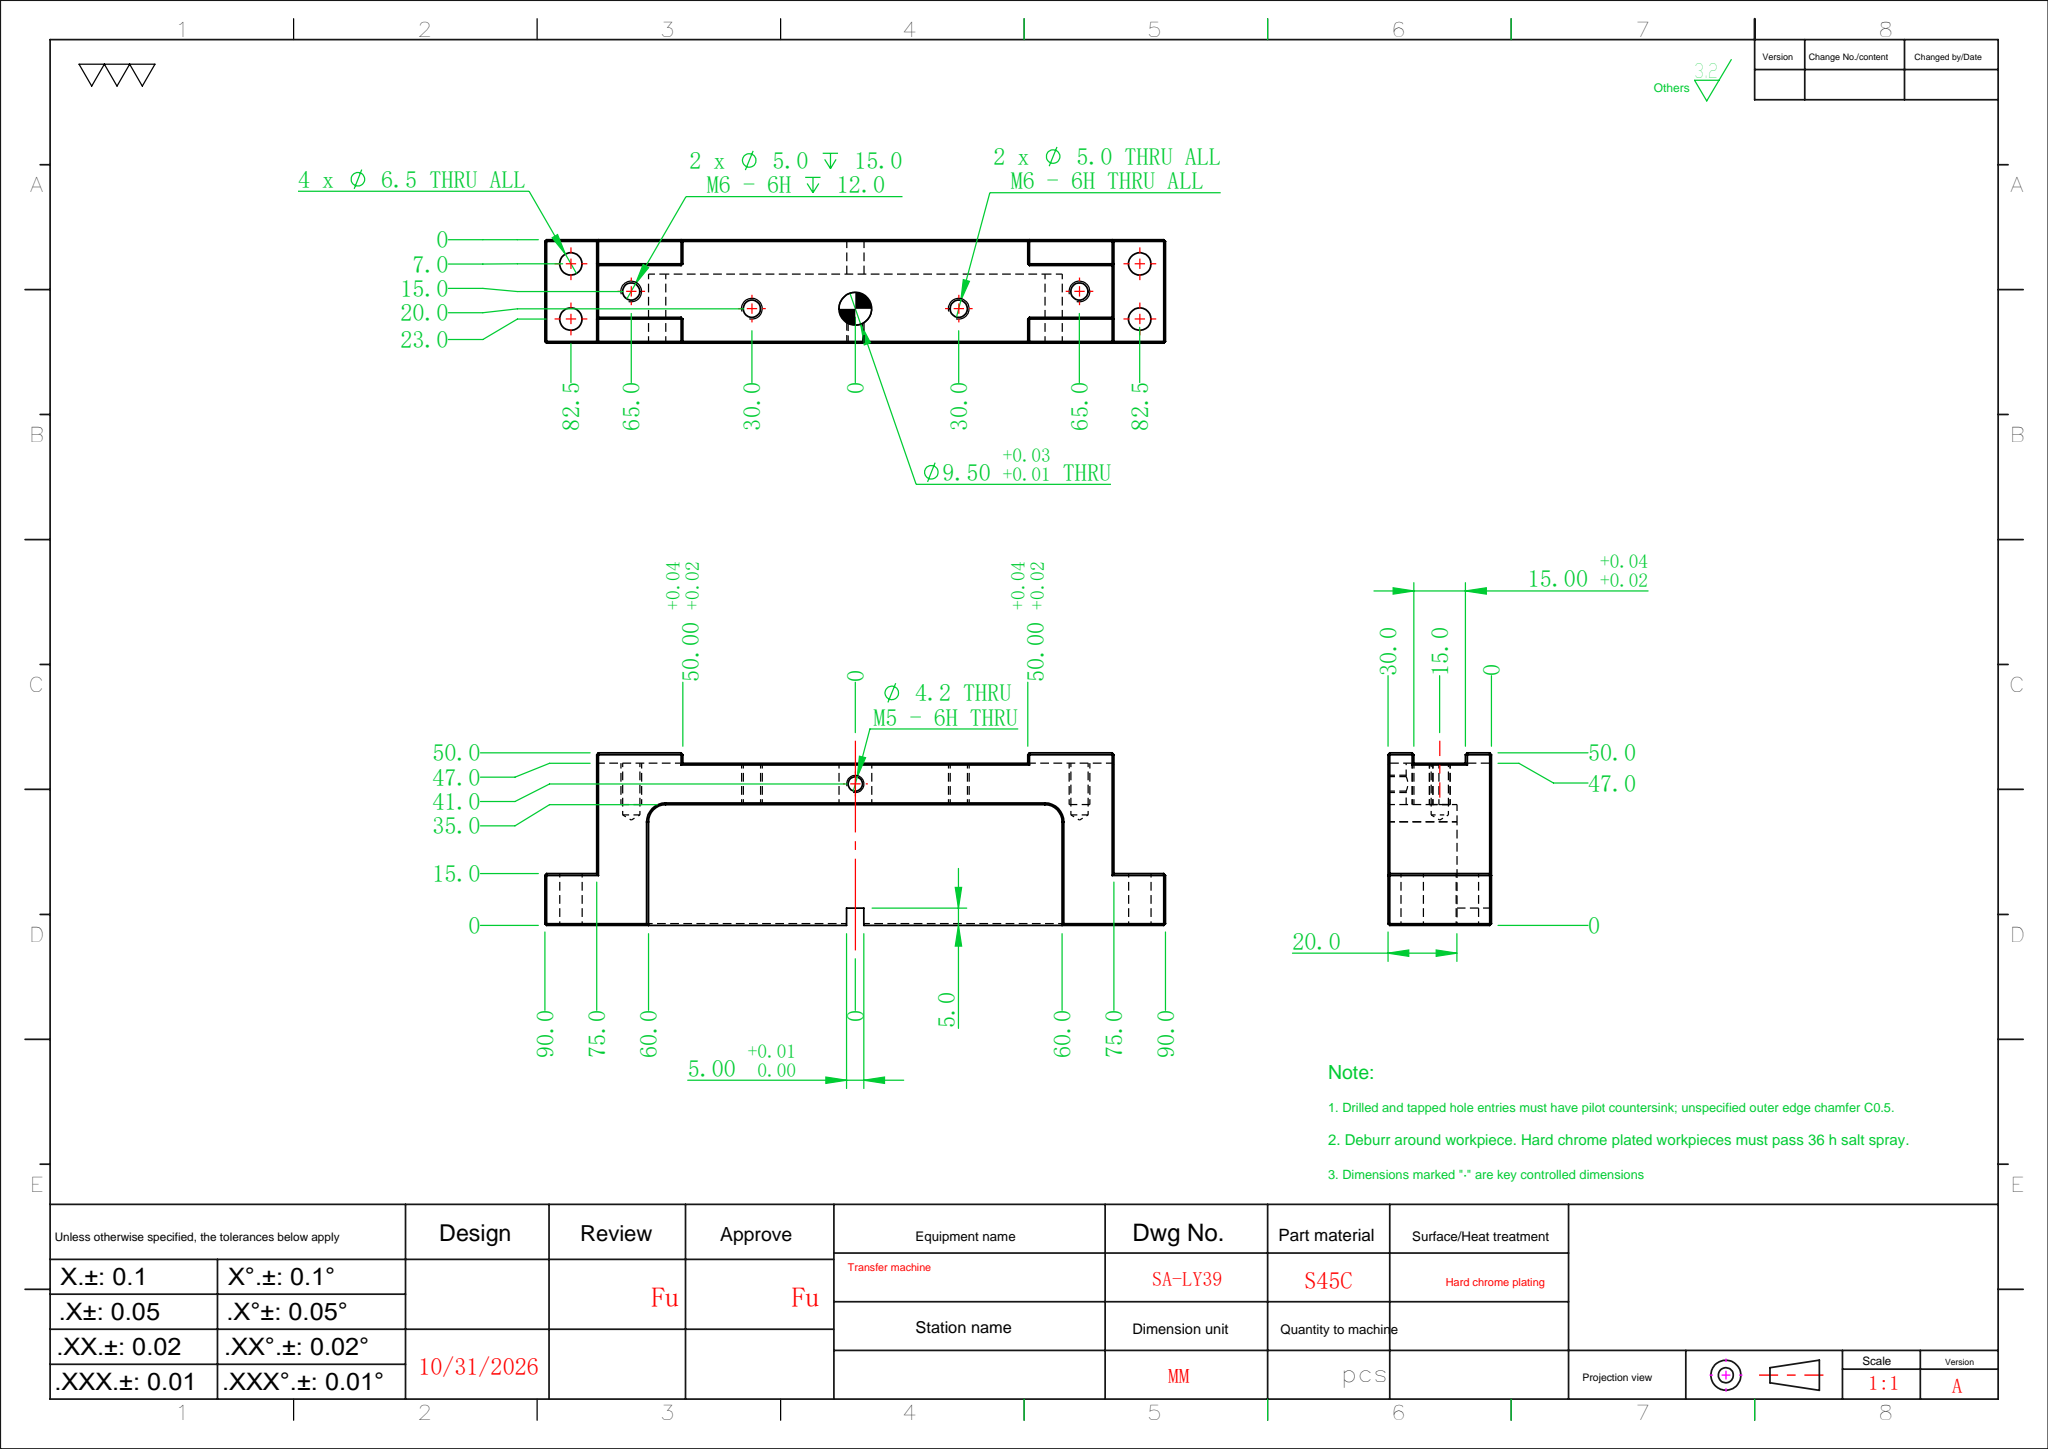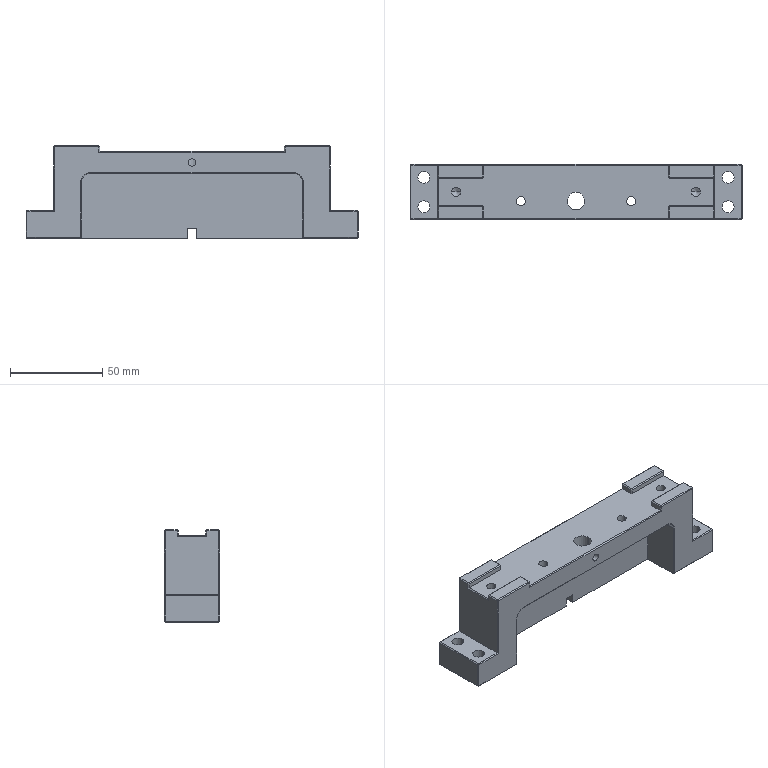Part | SolidWorks | features Cut 4, HoleWzd 4, ICE 2, Chamfer 1, Extrusion 1, Fillet 1 | 1 solid | 137 faces | box 180 x 30 x 50 mm | volume 139054 mm3 | plane 109 | cylinder 22 | cone 6 | commonest cylinder face diameters 5 x8 6.5 x8 4.2 x2 9.5 x2 10 x2